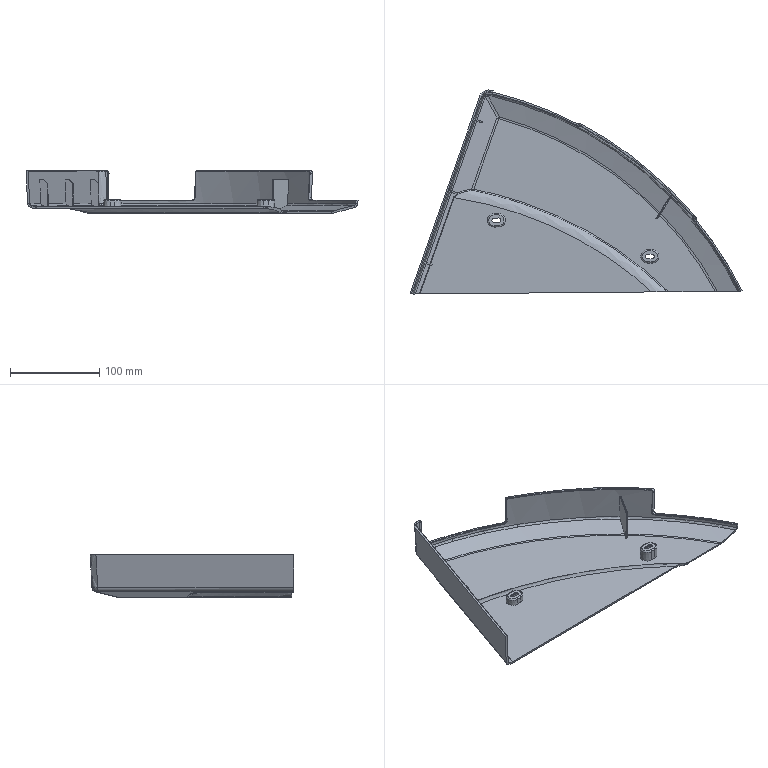Part | STEP file | Right column cover | 1 solid | 193 faces | box 372.789 x 229.022 x 48 mm | volume 179177 mm3 | plane 59 | spline 57 | cylinder 35 | cone 21 | torus 19 | sphere 2 | commonest cylinder face diameters 5 x6 6 x6 1.5 x5 4 x5 3 x4 1 x2